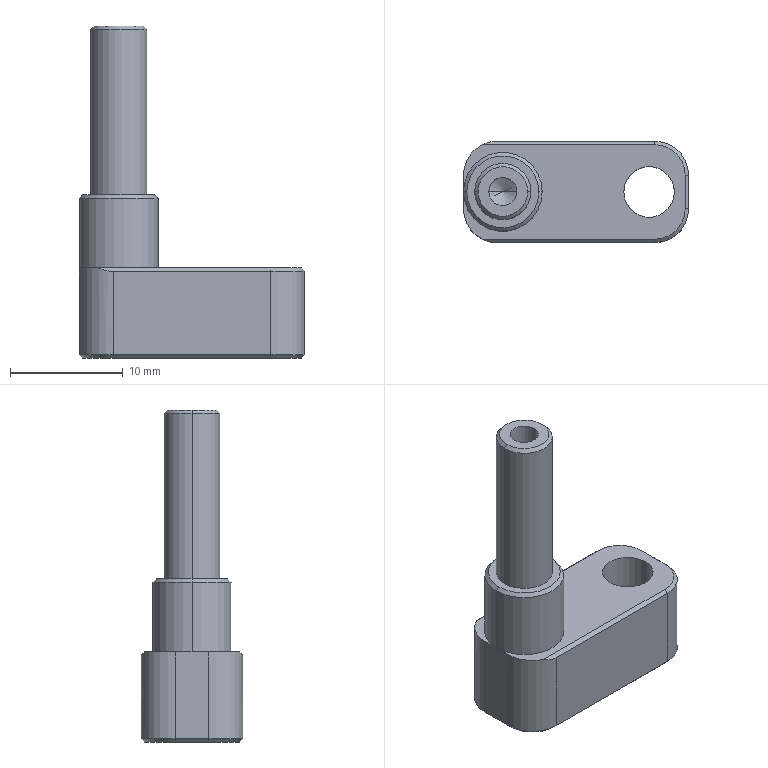Part | NX | features BREP 1 | 1 solid | 39 faces | box 20 x 9 x 29.5 mm | volume 1742 mm3 | plane 15 | cone 12 | cylinder 12 | commonest cylinder face diameters 6 x4 2.5 x2 4.5 x2 5 x2 7 x2
STEP:
#1=CARTESIAN_POINT('',(7.,4.2,8.));
#2=VERTEX_POINT('',#1);
#3=CARTESIAN_POINT('',(7.,4.5,7.7));
#4=VERTEX_POINT('',#3);
#5=CARTESIAN_POINT('',(7.,4.2,8.));
#6=DIRECTION('',(0.,0.7071,-0.7071));
#7=VECTOR('',#6,1000.);
#8=LINE('',#5,#7);
#9=EDGE_CURVE('',#2,#4,#8,.T.);
#10=ORIENTED_EDGE('',*,*,#9,.T.);
#11=CARTESIAN_POINT('',(-7.,4.5,7.7));
#12=VERTEX_POINT('',#11);
#13=CARTESIAN_POINT('',(7.,4.5,7.7));
#14=DIRECTION('',(1.,0.,0.));
#15=VECTOR('',#14,1000.);
#16=LINE('',#13,#15);
#17=EDGE_CURVE('',#12,#4,#16,.T.);
#18=ORIENTED_EDGE('',*,*,#17,.F.);
#19=CARTESIAN_POINT('',(-8.308,4.2,8.));
#20=VERTEX_POINT('',#19);
#21=CARTESIAN_POINT('',(-8.308,4.2,8.));
#22=CARTESIAN_POINT('',(-7.898,4.398,7.802));
#23=CARTESIAN_POINT('',(-7.455,4.5,7.7));
#24=CARTESIAN_POINT('',(-7.,4.5,7.7));
#25=(BOUNDED_CURVE()B_SPLINE_CURVE(3,(#21,#22,#23,#24),.UNSPECIFIED.,.F.,.F.)B_SPLINE_CURVE_WITH_KNOTS((4,4),(5.832,6.283),.UNSPECIFIED.)CURVE()GEOMETRIC_REPRESENTATION_ITEM()RATIONAL_B_SPLINE_CURVE((1.,0.9831,0.9831,1.))REPRESENTATION_ITEM(''));
#26=EDGE_CURVE('',#20,#12,#25,.T.);
#27=ORIENTED_EDGE('',*,*,#26,.F.);
#28=CARTESIAN_POINT('',(-7.,4.2,8.));
#29=DIRECTION('',(-1.,0.,0.));
#30=VECTOR('',#29,1000.);
#31=LINE('',#28,#30);
#32=EDGE_CURVE('',#2,#20,#31,.T.);
#33=ORIENTED_EDGE('',*,*,#32,.F.);
#34=EDGE_LOOP('',(#10,#18,#27,#33));
#35=FACE_BOUND('',#34,.T.);
#36=CARTESIAN_POINT('',(0.,4.2,8.));
#37=DIRECTION('',(0.,0.7071,0.7071));
#38=DIRECTION('',(1.,0.,0.));
#39=AXIS2_PLACEMENT_3D('',#36,#37,#38);
#40=PLANE('',#39);
#41=ADVANCED_FACE('',(#35),#40,.T.);
#42=CARTESIAN_POINT('',(9.7,1.5,8.));
#43=VERTEX_POINT('',#42);
#44=CARTESIAN_POINT('',(10.,1.5,7.7));
#45=VERTEX_POINT('',#44);
#46=CARTESIAN_POINT('',(9.7,1.5,8.));
#47=DIRECTION('',(0.7071,0.,-0.7071));
#48=VECTOR('',#47,1000.);
#49=LINE('',#46,#48);
#50=EDGE_CURVE('',#43,#45,#49,.T.);
#51=ORIENTED_EDGE('',*,*,#50,.T.);
#52=CARTESIAN_POINT('',(7.,1.5,7.7));
#53=DIRECTION('',(0.,0.,-1.));
#54=DIRECTION('',(1.,0.,0.));
#55=AXIS2_PLACEMENT_3D('',#52,#53,#54);
#56=CIRCLE('',#55,3.);
#57=EDGE_CURVE('',#4,#45,#56,.T.);
#58=ORIENTED_EDGE('',*,*,#57,.F.);
#59=ORIENTED_EDGE('',*,*,#9,.F.);
#60=CARTESIAN_POINT('',(7.,1.5,8.));
#61=DIRECTION('',(0.,0.,1.));
#62=DIRECTION('',(1.,0.,0.));
#63=AXIS2_PLACEMENT_3D('',#60,#61,#62);
#64=CIRCLE('',#63,2.7);
#65=EDGE_CURVE('',#43,#2,#64,.T.);
#66=ORIENTED_EDGE('',*,*,#65,.F.);
#67=EDGE_LOOP('',(#51,#58,#59,#66));
#68=FACE_BOUND('',#67,.T.);
#69=CARTESIAN_POINT('',(7.,1.5,8.));
#70=DIRECTION('',(0.,0.,-1.));
#71=DIRECTION('',(-1.,0.,0.));
#72=AXIS2_PLACEMENT_3D('',#69,#70,#71);
#73=CONICAL_SURFACE('',#72,2.7,0.7854);
#74=ADVANCED_FACE('',(#68),#73,.T.);
#75=CARTESIAN_POINT('',(9.7,-1.5,8.));
#76=VERTEX_POINT('',#75);
#77=CARTESIAN_POINT('',(10.,-1.5,7.7));
#78=VERTEX_POINT('',#77);
#79=CARTESIAN_POINT('',(9.7,-1.5,8.));
#80=DIRECTION('',(0.7071,0.,-0.7071));
#81=VECTOR('',#80,1000.);
#82=LINE('',#79,#81);
#83=EDGE_CURVE('',#76,#78,#82,.T.);
#84=ORIENTED_EDGE('',*,*,#83,.T.);
#85=CARTESIAN_POINT('',(10.,-1.5,7.7));
#86=DIRECTION('',(0.,-1.,0.));
#87=VECTOR('',#86,1000.);
#88=LINE('',#85,#87);
#89=EDGE_CURVE('',#45,#78,#88,.T.);
#90=ORIENTED_EDGE('',*,*,#89,.F.);
#91=ORIENTED_EDGE('',*,*,#50,.F.);
#92=CARTESIAN_POINT('',(9.7,1.5,8.));
#93=DIRECTION('',(0.,1.,0.));
#94=VECTOR('',#93,1000.);
#95=LINE('',#92,#94);
#96=EDGE_CURVE('',#76,#43,#95,.T.);
#97=ORIENTED_EDGE('',*,*,#96,.F.);
#98=EDGE_LOOP('',(#84,#90,#91,#97));
#99=FACE_BOUND('',#98,.T.);
#100=CARTESIAN_POINT('',(9.7,0.,8.));
#101=DIRECTION('',(0.7071,0.,0.7071));
#102=DIRECTION('',(0.,-1.,0.));
#103=AXIS2_PLACEMENT_3D('',#100,#101,#102);
#104=PLANE('',#103);
#105=ADVANCED_FACE('',(#99),#104,.T.);
#106=CARTESIAN_POINT('',(7.,-4.2,8.));
#107=VERTEX_POINT('',#106);
#108=CARTESIAN_POINT('',(7.,-4.5,7.7));
#109=VERTEX_POINT('',#108);
#110=CARTESIAN_POINT('',(7.,-4.2,8.));
#111=DIRECTION('',(0.,-0.7071,-0.7071));
#112=VECTOR('',#111,1000.);
#113=LINE('',#110,#112);
#114=EDGE_CURVE('',#107,#109,#113,.T.);
#115=ORIENTED_EDGE('',*,*,#114,.T.);
#116=CARTESIAN_POINT('',(7.,-1.5,7.7));
#117=DIRECTION('',(0.,0.,-1.));
#118=DIRECTION('',(1.,0.,0.));
#119=AXIS2_PLACEMENT_3D('',#116,#117,#118);
#120=CIRCLE('',#119,3.);
#121=EDGE_CURVE('',#78,#109,#120,.T.);
#122=ORIENTED_EDGE('',*,*,#121,.F.);
#123=ORIENTED_EDGE('',*,*,#83,.F.);
#124=CARTESIAN_POINT('',(7.,-1.5,8.));
#125=DIRECTION('',(0.,0.,1.));
#126=DIRECTION('',(1.,0.,0.));
#127=AXIS2_PLACEMENT_3D('',#124,#125,#126);
#128=CIRCLE('',#127,2.7);
#129=EDGE_CURVE('',#107,#76,#128,.T.);
#130=ORIENTED_EDGE('',*,*,#129,.F.);
#131=EDGE_LOOP('',(#115,#122,#123,#130));
#132=FACE_BOUND('',#131,.T.);
#133=CARTESIAN_POINT('',(7.,-1.5,8.));
#134=DIRECTION('',(0.,0.,-1.));
#135=DIRECTION('',(-1.,0.,0.));
#136=AXIS2_PLACEMENT_3D('',#133,#134,#135);
#137=CONICAL_SURFACE('',#136,2.7,0.7854);
#138=ADVANCED_FACE('',(#132),#137,.T.);
#139=CARTESIAN_POINT('',(-7.,-4.5,7.7));
#140=VERTEX_POINT('',#139);
#141=CARTESIAN_POINT('',(-8.308,-4.2,8.));
#142=VERTEX_POINT('',#141);
#143=CARTESIAN_POINT('',(-7.,-4.5,7.7));
#144=CARTESIAN_POINT('',(-7.455,-4.5,7.7));
#145=CARTESIAN_POINT('',(-7.898,-4.398,7.802));
#146=CARTESIAN_POINT('',(-8.308,-4.2,8.));
#147=(BOUNDED_CURVE()B_SPLINE_CURVE(3,(#143,#144,#145,#146),.UNSPECIFIED.,.F.,.F.)B_SPLINE_CURVE_WITH_KNOTS((4,4),(0.,0.451),.UNSPECIFIED.)CURVE()GEOMETRIC_REPRESENTATION_ITEM()RATIONAL_B_SPLINE_CURVE((1.,0.9831,0.9831,1.))REPRESENTATION_ITEM(''));
#148=EDGE_CURVE('',#140,#142,#147,.T.);
#149=ORIENTED_EDGE('',*,*,#148,.F.);
#150=CARTESIAN_POINT('',(-7.,-4.5,7.7));
#151=DIRECTION('',(-1.,0.,0.));
#152=VECTOR('',#151,1000.);
#153=LINE('',#150,#152);
#154=EDGE_CURVE('',#109,#140,#153,.T.);
#155=ORIENTED_EDGE('',*,*,#154,.F.);
#156=ORIENTED_EDGE('',*,*,#114,.F.);
#157=CARTESIAN_POINT('',(7.,-4.2,8.));
#158=DIRECTION('',(1.,0.,0.));
#159=VECTOR('',#158,1000.);
#160=LINE('',#157,#159);
#161=EDGE_CURVE('',#142,#107,#160,.T.);
#162=ORIENTED_EDGE('',*,*,#161,.F.);
#163=EDGE_LOOP('',(#149,#155,#156,#162));
#164=FACE_BOUND('',#163,.T.);
#165=CARTESIAN_POINT('',(0.,-4.2,8.));
#166=DIRECTION('',(0.,-0.7071,0.7071));
#167=DIRECTION('',(-1.,0.,0.));
#168=AXIS2_PLACEMENT_3D('',#165,#166,#167);
#169=PLANE('',#168);
#170=ADVANCED_FACE('',(#164),#169,.T.);
#171=CARTESIAN_POINT('',(-4.3,0.,29.5));
#172=VERTEX_POINT('',#171);
#173=CARTESIAN_POINT('',(-4.,0.,29.2));
#174=VERTEX_POINT('',#173);
#175=CARTESIAN_POINT('',(-4.3,0.,29.5));
#176=DIRECTION('',(0.7071,0.,-0.7071));
#177=VECTOR('',#176,1000.);
#178=LINE('',#175,#177);
#179=EDGE_CURVE('',#172,#174,#178,.T.);
#180=ORIENTED_EDGE('',*,*,#179,.F.);
#181=CARTESIAN_POINT('',(-8.7,0.,29.5));
#182=VERTEX_POINT('',#181);
#183=CARTESIAN_POINT('',(-6.5,0.,29.5));
#184=DIRECTION('',(0.,0.,1.));
#185=DIRECTION('',(1.,0.,0.));
#186=AXIS2_PLACEMENT_3D('',#183,#184,#185);
#187=CIRCLE('',#186,2.2);
#188=EDGE_CURVE('',#182,#172,#187,.T.);
#189=ORIENTED_EDGE('',*,*,#188,.F.);
#190=CARTESIAN_POINT('',(-9.,0.,29.2));
#191=VERTEX_POINT('',#190);
#192=CARTESIAN_POINT('',(-8.7,0.,29.5));
#193=DIRECTION('',(-0.7071,0.,-0.7071));
#194=VECTOR('',#193,1000.);
#195=LINE('',#192,#194);
#196=EDGE_CURVE('',#182,#191,#195,.T.);
#197=ORIENTED_EDGE('',*,*,#196,.T.);
#198=CARTESIAN_POINT('',(-6.5,0.,29.2));
#199=DIRECTION('',(0.,0.,-1.));
#200=DIRECTION('',(1.,0.,0.));
#201=AXIS2_PLACEMENT_3D('',#198,#199,#200);
#202=CIRCLE('',#201,2.5);
#203=EDGE_CURVE('',#174,#191,#202,.T.);
#204=ORIENTED_EDGE('',*,*,#203,.F.);
#205=EDGE_LOOP('',(#180,#189,#197,#204));
#206=FACE_BOUND('',#205,.T.);
#207=CARTESIAN_POINT('',(-6.5,0.,29.5));
#208=DIRECTION('',(0.,0.,-1.));
#209=DIRECTION('',(-1.,0.,0.));
#210=AXIS2_PLACEMENT_3D('',#207,#208,#209);
#211=CONICAL_SURFACE('',#210,2.2,0.7854);
#212=ADVANCED_FACE('',(#206),#211,.T.);
#213=CARTESIAN_POINT('',(-3.3,0.,14.5));
#214=VERTEX_POINT('',#213);
#215=CARTESIAN_POINT('',(-3.,0.,14.2));
#216=VERTEX_POINT('',#215);
#217=CARTESIAN_POINT('',(-3.3,0.,14.5));
#218=DIRECTION('',(0.7071,0.,-0.7071));
#219=VECTOR('',#218,1000.);
#220=LINE('',#217,#219);
#221=EDGE_CURVE('',#214,#216,#220,.T.);
#222=ORIENTED_EDGE('',*,*,#221,.F.);
#223=CARTESIAN_POINT('',(-9.7,0.,14.5));
#224=VERTEX_POINT('',#223);
#225=CARTESIAN_POINT('',(-6.5,0.,14.5));
#226=DIRECTION('',(0.,0.,1.));
#227=DIRECTION('',(1.,0.,0.));
#228=AXIS2_PLACEMENT_3D('',#225,#226,#227);
#229=CIRCLE('',#228,3.2);
#230=EDGE_CURVE('',#224,#214,#229,.T.);
#231=ORIENTED_EDGE('',*,*,#230,.F.);
#232=CARTESIAN_POINT('',(-10.,0.,14.2));
#233=VERTEX_POINT('',#232);
#234=CARTESIAN_POINT('',(-9.7,0.,14.5));
#235=DIRECTION('',(-0.7071,0.,-0.7071));
#236=VECTOR('',#235,1000.);
#237=LINE('',#234,#236);
#238=EDGE_CURVE('',#224,#233,#237,.T.);
#239=ORIENTED_EDGE('',*,*,#238,.T.);
#240=CARTESIAN_POINT('',(-6.5,0.,14.2));
#241=DIRECTION('',(0.,0.,-1.));
#242=DIRECTION('',(1.,0.,0.));
#243=AXIS2_PLACEMENT_3D('',#240,#241,#242);
#244=CIRCLE('',#243,3.5);
#245=EDGE_CURVE('',#216,#233,#244,.T.);
#246=ORIENTED_EDGE('',*,*,#245,.F.);
#247=EDGE_LOOP('',(#222,#231,#239,#246));
#248=FACE_BOUND('',#247,.T.);
#249=CARTESIAN_POINT('',(-6.5,0.,14.5));
#250=DIRECTION('',(0.,0.,-1.));
#251=DIRECTION('',(-1.,0.,0.));
#252=AXIS2_PLACEMENT_3D('',#249,#250,#251);
#253=CONICAL_SURFACE('',#252,3.2,0.7854);
#254=ADVANCED_FACE('',(#248),#253,.T.);
#255=CARTESIAN_POINT('',(7.,4.5,0.3));
#256=VERTEX_POINT('',#255);
#257=CARTESIAN_POINT('',(7.,4.2,0.));
#258=VERTEX_POINT('',#257);
#259=CARTESIAN_POINT('',(7.,4.5,0.3));
#260=DIRECTION('',(0.,-0.7071,-0.7071));
#261=VECTOR('',#260,1000.);
#262=LINE('',#259,#261);
#263=EDGE_CURVE('',#256,#258,#262,.T.);
#264=ORIENTED_EDGE('',*,*,#263,.T.);
#265=CARTESIAN_POINT('',(-7.,4.2,0.));
#266=VERTEX_POINT('',#265);
#267=CARTESIAN_POINT('',(0.,4.2,0.));
#268=DIRECTION('',(1.,0.,0.));
#269=VECTOR('',#268,1000.);
#270=LINE('',#267,#269);
#271=EDGE_CURVE('',#266,#258,#270,.T.);
#272=ORIENTED_EDGE('',*,*,#271,.F.);
#273=CARTESIAN_POINT('',(-7.,4.5,0.3));
#274=VERTEX_POINT('',#273);
#275=CARTESIAN_POINT('',(-7.,4.2,0.));
#276=DIRECTION('',(0.,0.7071,0.7071));
#277=VECTOR('',#276,1000.);
#278=LINE('',#275,#277);
#279=EDGE_CURVE('',#266,#274,#278,.T.);
#280=ORIENTED_EDGE('',*,*,#279,.T.);
#281=CARTESIAN_POINT('',(-10.,4.5,0.3));
#282=DIRECTION('',(-1.,0.,0.));
#283=VECTOR('',#282,1000.);
#284=LINE('',#281,#283);
#285=EDGE_CURVE('',#256,#274,#284,.T.);
#286=ORIENTED_EDGE('',*,*,#285,.F.);
#287=EDGE_LOOP('',(#264,#272,#280,#286));
#288=FACE_BOUND('',#287,.T.);
#289=CARTESIAN_POINT('',(-10.,4.5,0.3));
#290=DIRECTION('',(0.,-0.7071,0.7071));
#291=DIRECTION('',(-1.,0.,0.));
#292=AXIS2_PLACEMENT_3D('',#289,#290,#291);
#293=PLANE('',#292);
#294=ADVANCED_FACE('',(#288),#293,.F.);
#295=CARTESIAN_POINT('',(-9.7,1.5,0.));
#296=VERTEX_POINT('',#295);
#297=CARTESIAN_POINT('',(-10.,1.5,0.3));
#298=VERTEX_POINT('',#297);
#299=CARTESIAN_POINT('',(-9.7,1.5,0.));
#300=DIRECTION('',(-0.7071,0.,0.7071));
#301=VECTOR('',#300,1000.);
#302=LINE('',#299,#301);
#303=EDGE_CURVE('',#296,#298,#302,.T.);
#304=ORIENTED_EDGE('',*,*,#303,.T.);
#305=CARTESIAN_POINT('',(-7.,1.5,0.3));
#306=DIRECTION('',(0.,0.,1.));
#307=DIRECTION('',(1.,0.,0.));
#308=AXIS2_PLACEMENT_3D('',#305,#306,#307);
#309=CIRCLE('',#308,3.);
#310=EDGE_CURVE('',#274,#298,#309,.T.);
#311=ORIENTED_EDGE('',*,*,#310,.F.);
#312=ORIENTED_EDGE('',*,*,#279,.F.);
#313=CARTESIAN_POINT('',(-7.,1.5,0.));
#314=DIRECTION('',(0.,0.,-1.));
#315=DIRECTION('',(1.,0.,0.));
#316=AXIS2_PLACEMENT_3D('',#313,#314,#315);
#317=CIRCLE('',#316,2.7);
#318=EDGE_CURVE('',#296,#266,#317,.T.);
#319=ORIENTED_EDGE('',*,*,#318,.F.);
#320=EDGE_LOOP('',(#304,#311,#312,#319));
#321=FACE_BOUND('',#320,.T.);
#322=CARTESIAN_POINT('',(-7.,1.5,0.));
#323=DIRECTION('',(0.,0.,1.));
#324=DIRECTION('',(1.,0.,0.));
#325=AXIS2_PLACEMENT_3D('',#322,#323,#324);
#326=CONICAL_SURFACE('',#325,2.7,0.7854);
#327=ADVANCED_FACE('',(#321),#326,.T.);
#328=CARTESIAN_POINT('',(10.,1.5,0.3));
#329=VERTEX_POINT('',#328);
#330=CARTESIAN_POINT('',(9.7,1.5,0.));
#331=VERTEX_POINT('',#330);
#332=CARTESIAN_POINT('',(10.,1.5,0.3));
#333=DIRECTION('',(-0.7071,0.,-0.7071));
#334=VECTOR('',#333,1000.);
#335=LINE('',#332,#334);
#336=EDGE_CURVE('',#329,#331,#335,.T.);
#337=ORIENTED_EDGE('',*,*,#336,.T.);
#338=CARTESIAN_POINT('',(7.,1.5,0.));
#339=DIRECTION('',(0.,0.,-1.));
#340=DIRECTION('',(1.,0.,0.));
#341=AXIS2_PLACEMENT_3D('',#338,#339,#340);
#342=CIRCLE('',#341,2.7);
#343=EDGE_CURVE('',#258,#331,#342,.T.);
#344=ORIENTED_EDGE('',*,*,#343,.F.);
#345=ORIENTED_EDGE('',*,*,#263,.F.);
#346=CARTESIAN_POINT('',(7.,1.5,0.3));
#347=DIRECTION('',(0.,0.,1.));
#348=DIRECTION('',(1.,0.,0.));
#349=AXIS2_PLACEMENT_3D('',#346,#347,#348);
#350=CIRCLE('',#349,3.);
#351=EDGE_CURVE('',#329,#256,#350,.T.);
#352=ORIENTED_EDGE('',*,*,#351,.F.);
#353=EDGE_LOOP('',(#337,#344,#345,#352));
#354=FACE_BOUND('',#353,.T.);
#355=CARTESIAN_POINT('',(7.,1.5,0.));
#356=DIRECTION('',(0.,0.,1.));
#357=DIRECTION('',(1.,0.,0.));
#358=AXIS2_PLACEMENT_3D('',#355,#356,#357);
#359=CONICAL_SURFACE('',#358,2.7,0.7854);
#360=ADVANCED_FACE('',(#354),#359,.T.);
#361=CARTESIAN_POINT('',(-9.7,-1.5,0.));
#362=VERTEX_POINT('',#361);
#363=CARTESIAN_POINT('',(-10.,-1.5,0.3));
#364=VERTEX_POINT('',#363);
#365=CARTESIAN_POINT('',(-9.7,-1.5,0.));
#366=DIRECTION('',(-0.7071,0.,0.7071));
#367=VECTOR('',#366,1000.);
#368=LINE('',#365,#367);
#369=EDGE_CURVE('',#362,#364,#368,.T.);
#370=ORIENTED_EDGE('',*,*,#369,.T.);
#371=CARTESIAN_POINT('',(-10.,4.5,0.3));
#372=DIRECTION('',(0.,-1.,0.));
#373=VECTOR('',#372,1000.);
#374=LINE('',#371,#373);
#375=EDGE_CURVE('',#298,#364,#374,.T.);
#376=ORIENTED_EDGE('',*,*,#375,.F.);
#377=ORIENTED_EDGE('',*,*,#303,.F.);
#378=CARTESIAN_POINT('',(-9.7,0.,0.));
#379=DIRECTION('',(0.,1.,0.));
#380=VECTOR('',#379,1000.);
#381=LINE('',#378,#380);
#382=EDGE_CURVE('',#362,#296,#381,.T.);
#383=ORIENTED_EDGE('',*,*,#382,.F.);
#384=EDGE_LOOP('',(#370,#376,#377,#383));
#385=FACE_BOUND('',#384,.T.);
#386=CARTESIAN_POINT('',(-10.,4.5,0.3));
#387=DIRECTION('',(0.7071,0.,0.7071));
#388=DIRECTION('',(0.,-1.,0.));
#389=AXIS2_PLACEMENT_3D('',#386,#387,#388);
#390=PLANE('',#389);
#391=ADVANCED_FACE('',(#385),#390,.F.);
#392=CARTESIAN_POINT('',(10.,-1.5,0.3));
#393=VERTEX_POINT('',#392);
#394=CARTESIAN_POINT('',(9.7,-1.5,0.));
#395=VERTEX_POINT('',#394);
#396=CARTESIAN_POINT('',(10.,-1.5,0.3));
#397=DIRECTION('',(-0.7071,0.,-0.7071));
#398=VECTOR('',#397,1000.);
#399=LINE('',#396,#398);
#400=EDGE_CURVE('',#393,#395,#399,.T.);
#401=ORIENTED_EDGE('',*,*,#400,.T.);
#402=CARTESIAN_POINT('',(9.7,0.,0.));
#403=DIRECTION('',(0.,-1.,0.));
#404=VECTOR('',#403,1000.);
#405=LINE('',#402,#404);
#406=EDGE_CURVE('',#331,#395,#405,.T.);
#407=ORIENTED_EDGE('',*,*,#406,.F.);
#408=ORIENTED_EDGE('',*,*,#336,.F.);
#409=CARTESIAN_POINT('',(10.,4.5,0.3));
#410=DIRECTION('',(0.,1.,0.));
#411=VECTOR('',#410,1000.);
#412=LINE('',#409,#411);
#413=EDGE_CURVE('',#393,#329,#412,.T.);
#414=ORIENTED_EDGE('',*,*,#413,.F.);
#415=EDGE_LOOP('',(#401,#407,#408,#414));
#416=FACE_BOUND('',#415,.T.);
#417=CARTESIAN_POINT('',(10.,4.5,0.3));
#418=DIRECTION('',(-0.7071,0.,0.7071));
#419=DIRECTION('',(0.,1.,0.));
#420=AXIS2_PLACEMENT_3D('',#417,#418,#419);
#421=PLANE('',#420);
#422=ADVANCED_FACE('',(#416),#421,.F.);
#423=CARTESIAN_POINT('',(-7.,-4.2,0.));
#424=VERTEX_POINT('',#423);
#425=CARTESIAN_POINT('',(-7.,-4.5,0.3));
#426=VERTEX_POINT('',#425);
#427=CARTESIAN_POINT('',(-7.,-4.2,0.));
#428=DIRECTION('',(0.,-0.7071,0.7071));
#429=VECTOR('',#428,1000.);
#430=LINE('',#427,#429);
#431=EDGE_CURVE('',#424,#426,#430,.T.);
#432=ORIENTED_EDGE('',*,*,#431,.T.);
#433=CARTESIAN_POINT('',(-7.,-1.5,0.3));
#434=DIRECTION('',(0.,0.,1.));
#435=DIRECTION('',(1.,0.,0.));
#436=AXIS2_PLACEMENT_3D('',#433,#434,#435);
#437=CIRCLE('',#436,3.);
#438=EDGE_CURVE('',#364,#426,#437,.T.);
#439=ORIENTED_EDGE('',*,*,#438,.F.);
#440=ORIENTED_EDGE('',*,*,#369,.F.);
#441=CARTESIAN_POINT('',(-7.,-1.5,0.));
#442=DIRECTION('',(0.,0.,-1.));
#443=DIRECTION('',(1.,0.,0.));
#444=AXIS2_PLACEMENT_3D('',#441,#442,#443);
#445=CIRCLE('',#444,2.7);
#446=EDGE_CURVE('',#424,#362,#445,.T.);
#447=ORIENTED_EDGE('',*,*,#446,.F.);
#448=EDGE_LOOP('',(#432,#439,#440,#447));
#449=FACE_BOUND('',#448,.T.);
#450=CARTESIAN_POINT('',(-7.,-1.5,0.));
#451=DIRECTION('',(0.,0.,1.));
#452=DIRECTION('',(1.,0.,0.));
#453=AXIS2_PLACEMENT_3D('',#450,#451,#452);
#454=CONICAL_SURFACE('',#453,2.7,0.7854);
#455=ADVANCED_FACE('',(#449),#454,.T.);
#456=CARTESIAN_POINT('',(7.,-4.5,0.3));
#457=VERTEX_POINT('',#456);
#458=CARTESIAN_POINT('',(7.,-4.2,0.));
#459=VERTEX_POINT('',#458);
#460=CARTESIAN_POINT('',(7.,-4.5,0.3));
#461=DIRECTION('',(0.,0.7071,-0.7071));
#462=VECTOR('',#461,1000.);
#463=LINE('',#460,#462);
#464=EDGE_CURVE('',#457,#459,#463,.T.);
#465=ORIENTED_EDGE('',*,*,#464,.T.);
#466=CARTESIAN_POINT('',(7.,-1.5,0.));
#467=DIRECTION('',(0.,0.,-1.));
#468=DIRECTION('',(1.,0.,0.));
#469=AXIS2_PLACEMENT_3D('',#466,#467,#468);
#470=CIRCLE('',#469,2.7);
#471=EDGE_CURVE('',#395,#459,#470,.T.);
#472=ORIENTED_EDGE('',*,*,#471,.F.);
#473=ORIENTED_EDGE('',*,*,#400,.F.);
#474=CARTESIAN_POINT('',(7.,-1.5,0.3));
#475=DIRECTION('',(0.,0.,1.));
#476=DIRECTION('',(1.,0.,0.));
#477=AXIS2_PLACEMENT_3D('',#474,#475,#476);
#478=CIRCLE('',#477,3.);
#479=EDGE_CURVE('',#457,#393,#478,.T.);
#480=ORIENTED_EDGE('',*,*,#479,.F.);
#481=EDGE_LOOP('',(#465,#472,#473,#480));
#482=FACE_BOUND('',#481,.T.);
#483=CARTESIAN_POINT('',(7.,-1.5,0.));
#484=DIRECTION('',(0.,0.,1.));
#485=DIRECTION('',(1.,0.,0.));
#486=AXIS2_PLACEMENT_3D('',#483,#484,#485);
#487=CONICAL_SURFACE('',#486,2.7,0.7854);
#488=ADVANCED_FACE('',(#482),#487,.T.);
#489=ORIENTED_EDGE('',*,*,#431,.F.);
#490=CARTESIAN_POINT('',(0.,-4.2,0.));
#491=DIRECTION('',(-1.,0.,0.));
#492=VECTOR('',#491,1000.);
#493=LINE('',#490,#492);
#494=EDGE_CURVE('',#459,#424,#493,.T.);
#495=ORIENTED_EDGE('',*,*,#494,.F.);
#496=ORIENTED_EDGE('',*,*,#464,.F.);
#497=CARTESIAN_POINT('',(-10.,-4.5,0.3));
#498=DIRECTION('',(1.,0.,0.));
#499=VECTOR('',#498,1000.);
#500=LINE('',#497,#499);
#501=EDGE_CURVE('',#426,#457,#500,.T.);
#502=ORIENTED_EDGE('',*,*,#501,.F.);
#503=EDGE_LOOP('',(#489,#495,#496,#502));
#504=FACE_BOUND('',#503,.T.);
#505=CARTESIAN_POINT('',(-10.,-4.5,0.3));
#506=DIRECTION('',(0.,0.7071,0.7071));
#507=DIRECTION('',(1.,0.,0.));
#508=AXIS2_PLACEMENT_3D('',#505,#506,#507);
#509=PLANE('',#508);
#510=ADVANCED_FACE('',(#504),#509,.F.);
#511=CARTESIAN_POINT('',(-7.,-4.5,8.));
#512=DIRECTION('',(0.,0.,-1.));
#513=VECTOR('',#512,1000.);
#514=LINE('',#511,#513);
#515=EDGE_CURVE('',#140,#426,#514,.T.);
#516=ORIENTED_EDGE('',*,*,#515,.F.);
#517=ORIENTED_EDGE('',*,*,#148,.T.);
#518=CARTESIAN_POINT('',(-10.,-1.5,8.));
#519=VERTEX_POINT('',#518);
#520=CARTESIAN_POINT('',(-7.,-1.5,8.));
#521=DIRECTION('',(0.,0.,1.));
#522=DIRECTION('',(1.,0.,0.));
#523=AXIS2_PLACEMENT_3D('',#520,#521,#522);
#524=CIRCLE('',#523,3.);
#525=EDGE_CURVE('',#519,#142,#524,.T.);
#526=ORIENTED_EDGE('',*,*,#525,.F.);
#527=CARTESIAN_POINT('',(-10.,-1.5,8.));
#528=DIRECTION('',(0.,0.,1.));
#529=VECTOR('',#528,1000.);
#530=LINE('',#527,#529);
#531=EDGE_CURVE('',#364,#519,#530,.T.);
#532=ORIENTED_EDGE('',*,*,#531,.F.);
#533=ORIENTED_EDGE('',*,*,#438,.T.);
#534=EDGE_LOOP('',(#516,#517,#526,#532,#533));
#535=FACE_BOUND('',#534,.T.);
#536=CARTESIAN_POINT('',(-7.,-1.5,8.));
#537=DIRECTION('',(0.,0.,-1.));
#538=DIRECTION('',(-1.,0.,0.));
#539=AXIS2_PLACEMENT_3D('',#536,#537,#538);
#540=CYLINDRICAL_SURFACE('',#539,3.);
#541=ADVANCED_FACE('',(#535),#540,.T.);
#542=CARTESIAN_POINT('',(10.,-1.5,8.));
#543=DIRECTION('',(0.,0.,-1.));
#544=VECTOR('',#543,1000.);
#545=LINE('',#542,#544);
#546=EDGE_CURVE('',#78,#393,#545,.T.);
#547=ORIENTED_EDGE('',*,*,#546,.F.);
#548=ORIENTED_EDGE('',*,*,#121,.T.);
#549=CARTESIAN_POINT('',(7.,-4.5,8.));
#550=DIRECTION('',(0.,0.,1.));
#551=VECTOR('',#550,1000.);
#552=LINE('',#549,#551);
#553=EDGE_CURVE('',#457,#109,#552,.T.);
#554=ORIENTED_EDGE('',*,*,#553,.F.);
#555=ORIENTED_EDGE('',*,*,#479,.T.);
#556=EDGE_LOOP('',(#547,#548,#554,#555));
#557=FACE_BOUND('',#556,.T.);
#558=CARTESIAN_POINT('',(7.,-1.5,8.));
#559=DIRECTION('',(0.,0.,-1.));
#560=DIRECTION('',(-1.,0.,0.));
#561=AXIS2_PLACEMENT_3D('',#558,#559,#560);
#562=CYLINDRICAL_SURFACE('',#561,3.);
#563=ADVANCED_FACE('',(#557),#562,.T.);
#564=CARTESIAN_POINT('',(7.,4.5,8.));
#565=DIRECTION('',(0.,0.,-1.));
#566=VECTOR('',#565,1000.);
#567=LINE('',#564,#566);
#568=EDGE_CURVE('',#4,#256,#567,.T.);
#569=ORIENTED_EDGE('',*,*,#568,.F.);
#570=ORIENTED_EDGE('',*,*,#57,.T.);
#571=CARTESIAN_POINT('',(10.,1.5,8.));
#572=DIRECTION('',(0.,0.,1.));
#573=VECTOR('',#572,1000.);
#574=LINE('',#571,#573);
#575=EDGE_CURVE('',#329,#45,#574,.T.);
#576=ORIENTED_EDGE('',*,*,#575,.F.);
#577=ORIENTED_EDGE('',*,*,#351,.T.);
#578=EDGE_LOOP('',(#569,#570,#576,#577));
#579=FACE_BOUND('',#578,.T.);
#580=CARTESIAN_POINT('',(7.,1.5,8.));
#581=DIRECTION('',(0.,0.,-1.));
#582=DIRECTION('',(-1.,0.,0.));
#583=AXIS2_PLACEMENT_3D('',#580,#581,#582);
#584=CYLINDRICAL_SURFACE('',#583,3.);
#585=ADVANCED_FACE('',(#579),#584,.T.);
#586=CARTESIAN_POINT('',(-10.,1.5,8.));
#587=VERTEX_POINT('',#586);
#588=CARTESIAN_POINT('',(-7.,1.5,8.));
#589=DIRECTION('',(0.,0.,1.));
#590=DIRECTION('',(1.,0.,0.));
#591=AXIS2_PLACEMENT_3D('',#588,#589,#590);
#592=CIRCLE('',#591,3.);
#593=EDGE_CURVE('',#20,#587,#592,.T.);
#594=ORIENTED_EDGE('',*,*,#593,.F.);
#595=ORIENTED_EDGE('',*,*,#26,.T.);
#596=CARTESIAN_POINT('',(-7.,4.5,8.));
#597=DIRECTION('',(0.,0.,1.));
#598=VECTOR('',#597,1000.);
#599=LINE('',#596,#598);
#600=EDGE_CURVE('',#274,#12,#599,.T.);
#601=ORIENTED_EDGE('',*,*,#600,.F.);
#602=ORIENTED_EDGE('',*,*,#310,.T.);
#603=CARTESIAN_POINT('',(-10.,1.5,8.));
#604=DIRECTION('',(0.,0.,-1.));
#605=VECTOR('',#604,1000.);
#606=LINE('',#603,#605);
#607=EDGE_CURVE('',#587,#298,#606,.T.);
#608=ORIENTED_EDGE('',*,*,#607,.F.);
#609=EDGE_LOOP('',(#594,#595,#601,#602,#608));
#610=FACE_BOUND('',#609,.T.);
#611=CARTESIAN_POINT('',(-7.,1.5,8.));
#612=DIRECTION('',(0.,0.,-1.));
#613=DIRECTION('',(-1.,0.,0.));
#614=AXIS2_PLACEMENT_3D('',#611,#612,#613);
#615=CYLINDRICAL_SURFACE('',#614,3.);
#616=ADVANCED_FACE('',(#610),#615,.T.);
#617=CARTESIAN_POINT('',(-7.75,0.,29.5));
#618=VERTEX_POINT('',#617);
#619=CARTESIAN_POINT('',(-7.75,0.,20.));
#620=VERTEX_POINT('',#619);
#621=CARTESIAN_POINT('',(-7.75,0.,29.5));
#622=DIRECTION('',(0.,0.,1.));
#623=VECTOR('',#622,1000.);
#624=LINE('',#621,#623);
#625=EDGE_CURVE('',#618,#620,#624,.F.);
#626=ORIENTED_EDGE('',*,*,#625,.T.);
#627=CARTESIAN_POINT('',(-5.25,0.,20.));
#628=VERTEX_POINT('',#627);
#629=CARTESIAN_POINT('',(-6.5,0.,20.));
#630=DIRECTION('',(0.,0.,1.));
#631=DIRECTION('',(1.,0.,0.));
#632=AXIS2_PLACEMENT_3D('',#629,#630,#631);
#633=CIRCLE('',#632,1.25);
#634=EDGE_CURVE('',#628,#620,#633,.T.);
#635=ORIENTED_EDGE('',*,*,#634,.F.);
#636=CARTESIAN_POINT('',(-5.25,0.,29.5));
#637=VERTEX_POINT('',#636);
#638=CARTESIAN_POINT('',(-5.25,0.,29.5));
#639=DIRECTION('',(0.,0.,1.));
#640=VECTOR('',#639,1000.);
#641=LINE('',#638,#640);
#642=EDGE_CURVE('',#637,#628,#641,.F.);
#643=ORIENTED_EDGE('',*,*,#642,.F.);
#644=CARTESIAN_POINT('',(-6.5,0.,29.5));
#645=DIRECTION('',(0.,0.,1.));
#646=DIRECTION('',(1.,0.,0.));
#647=AXIS2_PLACEMENT_3D('',#644,#645,#646);
#648=CIRCLE('',#647,1.25);
#649=EDGE_CURVE('',#637,#618,#648,.T.);
#650=ORIENTED_EDGE('',*,*,#649,.T.);
#651=EDGE_LOOP('',(#626,#635,#643,#650));
#652=FACE_BOUND('',#651,.T.);
#653=CARTESIAN_POINT('',(-6.5,0.,29.5));
#654=DIRECTION('',(0.,0.,1.));
#655=DIRECTION('',(1.,0.,0.));
#656=AXIS2_PLACEMENT_3D('',#653,#654,#655);
#657=CYLINDRICAL_SURFACE('',#656,1.25);
#658=ADVANCED_FACE('',(#652),#657,.F.);
#659=CARTESIAN_POINT('',(-6.5,0.,19.249));
#660=VERTEX_POINT('',#659);
#661=CARTESIAN_POINT('',(-7.75,0.,20.));
#662=DIRECTION('',(-0.8572,0.,0.515));
#663=VECTOR('',#662,1000.);
#664=LINE('',#661,#663);
#665=EDGE_CURVE('',#660,#620,#664,.T.);
#666=ORIENTED_EDGE('',*,*,#665,.F.);
#667=CARTESIAN_POINT('',(-5.25,0.,20.));
#668=DIRECTION('',(0.8572,0.,0.515));
#669=VECTOR('',#668,1000.);
#670=LINE('',#667,#669);
#671=EDGE_CURVE('',#660,#628,#670,.T.);
#672=ORIENTED_EDGE('',*,*,#671,.T.);
#673=ORIENTED_EDGE('',*,*,#634,.T.);
#674=EDGE_LOOP('',(#666,#672,#673));
#675=FACE_BOUND('',#674,.T.);
#676=CARTESIAN_POINT('',(-6.5,0.,20.));
#677=DIRECTION('',(0.,0.,1.));
#678=DIRECTION('',(1.,0.,0.));
#679=AXIS2_PLACEMENT_3D('',#676,#677,#678);
#680=CONICAL_SURFACE('',#679,1.25,1.03);
#681=ADVANCED_FACE('',(#675),#680,.F.);
#682=CARTESIAN_POINT('',(4.25,0.,8.));
#683=VERTEX_POINT('',#682);
#684=CARTESIAN_POINT('',(4.25,0.,0.));
#685=VERTEX_POINT('',#684);
#686=CARTESIAN_POINT('',(4.25,0.,-7.));
#687=DIRECTION('',(0.,0.,1.));
#688=VECTOR('',#687,1000.);
#689=LINE('',#686,#688);
#690=EDGE_CURVE('',#683,#685,#689,.F.);
#691=ORIENTED_EDGE('',*,*,#690,.T.);
#692=CARTESIAN_POINT('',(8.75,0.,0.));
#693=VERTEX_POINT('',#692);
#694=CARTESIAN_POINT('',(6.5,0.,0.));
#695=DIRECTION('',(0.,0.,1.));
#696=DIRECTION('',(1.,0.,0.));
#697=AXIS2_PLACEMENT_3D('',#694,#695,#696);
#698=CIRCLE('',#697,2.25);
#699=EDGE_CURVE('',#693,#685,#698,.T.);
#700=ORIENTED_EDGE('',*,*,#699,.F.);
#701=CARTESIAN_POINT('',(8.75,0.,8.));
#702=VERTEX_POINT('',#701);
#703=CARTESIAN_POINT('',(8.75,0.,-7.));
#704=DIRECTION('',(0.,0.,1.));
#705=VECTOR('',#704,1000.);
#706=LINE('',#703,#705);
#707=EDGE_CURVE('',#702,#693,#706,.F.);
#708=ORIENTED_EDGE('',*,*,#707,.F.);
#709=CARTESIAN_POINT('',(6.5,0.,8.));
#710=DIRECTION('',(0.,0.,1.));
#711=DIRECTION('',(1.,0.,0.));
#712=AXIS2_PLACEMENT_3D('',#709,#710,#711);
#713=CIRCLE('',#712,2.25);
#714=EDGE_CURVE('',#702,#683,#713,.T.);
#715=ORIENTED_EDGE('',*,*,#714,.T.);
#716=EDGE_LOOP('',(#691,#700,#708,#715));
#717=FACE_BOUND('',#716,.T.);
#718=CARTESIAN_POINT('',(6.5,0.,-7.));
#719=DIRECTION('',(0.,0.,1.));
#720=DIRECTION('',(1.,0.,0.));
#721=AXIS2_PLACEMENT_3D('',#718,#719,#720);
#722=CYLINDRICAL_SURFACE('',#721,2.25);
#723=ADVANCED_FACE('',(#717),#722,.F.);
#724=ORIENTED_EDGE('',*,*,#649,.F.);
#725=CARTESIAN_POINT('',(-6.5,0.,29.5));
#726=DIRECTION('',(0.,0.,1.));
#727=DIRECTION('',(1.,0.,0.));
#728=AXIS2_PLACEMENT_3D('',#725,#726,#727);
#729=CIRCLE('',#728,1.25);
#730=EDGE_CURVE('',#618,#637,#729,.T.);
#731=ORIENTED_EDGE('',*,*,#730,.F.);
#732=EDGE_LOOP('',(#724,#731));
#733=FACE_BOUND('',#732,.T.);
#734=ORIENTED_EDGE('',*,*,#188,.T.);
#735=CARTESIAN_POINT('',(-6.5,0.,29.5));
#736=DIRECTION('',(0.,0.,1.));
#737=DIRECTION('',(1.,0.,0.));
#738=AXIS2_PLACEMENT_3D('',#735,#736,#737);
#739=CIRCLE('',#738,2.2);
#740=EDGE_CURVE('',#172,#182,#739,.T.);
#741=ORIENTED_EDGE('',*,*,#740,.T.);
#742=EDGE_LOOP('',(#734,#741));
#743=FACE_BOUND('',#742,.T.);
#744=CARTESIAN_POINT('',(-6.5,0.,29.5));
#745=DIRECTION('',(0.,0.,1.));
#746=DIRECTION('',(1.,0.,0.));
#747=AXIS2_PLACEMENT_3D('',#744,#745,#746);
#748=PLANE('',#747);
#749=ADVANCED_FACE('',(#733,#743),#748,.T.);
#750=CARTESIAN_POINT('',(-4.,0.,14.5));
#751=VERTEX_POINT('',#750);
#752=CARTESIAN_POINT('',(-4.,0.,29.5));
#753=DIRECTION('',(0.,0.,-1.));
#754=VECTOR('',#753,1000.);
#755=LINE('',#752,#754);
#756=EDGE_CURVE('',#174,#751,#755,.T.);
#757=ORIENTED_EDGE('',*,*,#756,.F.);
#758=ORIENTED_EDGE('',*,*,#203,.T.);
#759=CARTESIAN_POINT('',(-9.,0.,14.5));
#760=VERTEX_POINT('',#759);
#761=CARTESIAN_POINT('',(-9.,0.,29.5));
#762=DIRECTION('',(0.,0.,-1.));
#763=VECTOR('',#762,1000.);
#764=LINE('',#761,#763);
#765=EDGE_CURVE('',#191,#760,#764,.T.);
#766=ORIENTED_EDGE('',*,*,#765,.T.);
#767=CARTESIAN_POINT('',(-6.5,0.,14.5));
#768=DIRECTION('',(0.,0.,1.));
#769=DIRECTION('',(1.,0.,0.));
#770=AXIS2_PLACEMENT_3D('',#767,#768,#769);
#771=CIRCLE('',#770,2.5);
#772=EDGE_CURVE('',#760,#751,#771,.T.);
#773=ORIENTED_EDGE('',*,*,#772,.T.);
#774=EDGE_LOOP('',(#757,#758,#766,#773));
#775=FACE_BOUND('',#774,.T.);
#776=CARTESIAN_POINT('',(-6.5,0.,29.5));
#777=DIRECTION('',(0.,0.,-1.));
#778=DIRECTION('',(-1.,0.,0.));
#779=AXIS2_PLACEMENT_3D('',#776,#777,#778);
#780=CYLINDRICAL_SURFACE('',#779,2.5);
#781=ADVANCED_FACE('',(#775),#780,.T.);
#782=ORIENTED_EDGE('',*,*,#772,.F.);
#783=CARTESIAN_POINT('',(-6.5,0.,14.5));
#784=DIRECTION('',(0.,0.,1.));
#785=DIRECTION('',(1.,0.,0.));
#786=AXIS2_PLACEMENT_3D('',#783,#784,#785);
#787=CIRCLE('',#786,2.5);
#788=EDGE_CURVE('',#751,#760,#787,.T.);
#789=ORIENTED_EDGE('',*,*,#788,.F.);
#790=EDGE_LOOP('',(#782,#789));
#791=FACE_BOUND('',#790,.T.);
#792=ORIENTED_EDGE('',*,*,#230,.T.);
#793=CARTESIAN_POINT('',(-6.5,0.,14.5));
#794=DIRECTION('',(0.,0.,1.));
#795=DIRECTION('',(1.,0.,0.));
#796=AXIS2_PLACEMENT_3D('',#793,#794,#795);
#797=CIRCLE('',#796,3.2);
#798=EDGE_CURVE('',#214,#224,#797,.T.);
#799=ORIENTED_EDGE('',*,*,#798,.T.);
#800=EDGE_LOOP('',(#792,#799));
#801=FACE_BOUND('',#800,.T.);
#802=CARTESIAN_POINT('',(-6.5,0.,14.5));
#803=DIRECTION('',(0.,0.,1.));
#804=DIRECTION('',(1.,0.,0.));
#805=AXIS2_PLACEMENT_3D('',#802,#803,#804);
#806=PLANE('',#805);
#807=ADVANCED_FACE('',(#791,#801),#806,.T.);
#808=CARTESIAN_POINT('',(-3.,0.,8.));
#809=VERTEX_POINT('',#808);
#810=CARTESIAN_POINT('',(-3.,0.,14.5));
#811=DIRECTION('',(0.,0.,-1.));
#812=VECTOR('',#811,1000.);
#813=LINE('',#810,#812);
#814=EDGE_CURVE('',#216,#809,#813,.T.);
#815=ORIENTED_EDGE('',*,*,#814,.F.);
#816=ORIENTED_EDGE('',*,*,#245,.T.);
#817=CARTESIAN_POINT('',(-10.,0.,8.));
#818=VERTEX_POINT('',#817);
#819=CARTESIAN_POINT('',(-10.,0.,14.5));
#820=DIRECTION('',(0.,0.,-1.));
#821=VECTOR('',#820,1000.);
#822=LINE('',#819,#821);
#823=EDGE_CURVE('',#233,#818,#822,.T.);
#824=ORIENTED_EDGE('',*,*,#823,.T.);
#825=CARTESIAN_POINT('',(-6.5,0.,8.));
#826=DIRECTION('',(0.,0.,1.));
#827=DIRECTION('',(1.,0.,0.));
#828=AXIS2_PLACEMENT_3D('',#825,#826,#827);
#829=CIRCLE('',#828,3.5);
#830=EDGE_CURVE('',#818,#809,#829,.T.);
#831=ORIENTED_EDGE('',*,*,#830,.T.);
#832=EDGE_LOOP('',(#815,#816,#824,#831));
#833=FACE_BOUND('',#832,.T.);
#834=CARTESIAN_POINT('',(-6.5,0.,14.5));
#835=DIRECTION('',(0.,0.,-1.));
#836=DIRECTION('',(-1.,0.,0.));
#837=AXIS2_PLACEMENT_3D('',#834,#835,#836);
#838=CYLINDRICAL_SURFACE('',#837,3.5);
#839=ADVANCED_FACE('',(#833),#838,.T.);
#840=ORIENTED_EDGE('',*,*,#699,.T.);
#841=CARTESIAN_POINT('',(6.5,0.,0.));
#842=DIRECTION('',(0.,0.,1.));
#843=DIRECTION('',(1.,0.,0.));
#844=AXIS2_PLACEMENT_3D('',#841,#842,#843);
#845=CIRCLE('',#844,2.25);
#846=EDGE_CURVE('',#685,#693,#845,.T.);
#847=ORIENTED_EDGE('',*,*,#846,.T.);
#848=EDGE_LOOP('',(#840,#847));
#849=FACE_BOUND('',#848,.T.);
#850=ORIENTED_EDGE('',*,*,#318,.T.);
#851=ORIENTED_EDGE('',*,*,#271,.T.);
#852=ORIENTED_EDGE('',*,*,#343,.T.);
#853=ORIENTED_EDGE('',*,*,#406,.T.);
#854=ORIENTED_EDGE('',*,*,#471,.T.);
#855=ORIENTED_EDGE('',*,*,#494,.T.);
#856=ORIENTED_EDGE('',*,*,#446,.T.);
#857=ORIENTED_EDGE('',*,*,#382,.T.);
#858=EDGE_LOOP('',(#850,#851,#852,#853,#854,#855,#856,#857));
#859=FACE_BOUND('',#858,.T.);
#860=CARTESIAN_POINT('',(0.,0.,0.));
#861=DIRECTION('',(0.,0.,1.));
#862=DIRECTION('',(1.,0.,0.));
#863=AXIS2_PLACEMENT_3D('',#860,#861,#862);
#864=PLANE('',#863);
#865=ADVANCED_FACE('',(#849,#859),#864,.F.);
#866=ORIENTED_EDGE('',*,*,#65,.T.);
#867=ORIENTED_EDGE('',*,*,#32,.T.);
#868=ORIENTED_EDGE('',*,*,#593,.T.);
#869=CARTESIAN_POINT('',(-10.,4.5,8.));
#870=DIRECTION('',(0.,-1.,0.));
#871=VECTOR('',#870,1000.);
#872=LINE('',#869,#871);
#873=EDGE_CURVE('',#587,#818,#872,.T.);
#874=ORIENTED_EDGE('',*,*,#873,.T.);
#875=CARTESIAN_POINT('',(-6.5,0.,8.));
#876=DIRECTION('',(0.,0.,1.));
#877=DIRECTION('',(1.,0.,0.));
#878=AXIS2_PLACEMENT_3D('',#875,#876,#877);
#879=CIRCLE('',#878,3.5);
#880=EDGE_CURVE('',#809,#818,#879,.T.);
#881=ORIENTED_EDGE('',*,*,#880,.F.);
#882=ORIENTED_EDGE('',*,*,#830,.F.);
#883=CARTESIAN_POINT('',(-10.,4.5,8.));
#884=DIRECTION('',(0.,-1.,0.));
#885=VECTOR('',#884,1000.);
#886=LINE('',#883,#885);
#887=EDGE_CURVE('',#818,#519,#886,.T.);
#888=ORIENTED_EDGE('',*,*,#887,.T.);
#889=ORIENTED_EDGE('',*,*,#525,.T.);
#890=ORIENTED_EDGE('',*,*,#161,.T.);
#891=ORIENTED_EDGE('',*,*,#129,.T.);
#892=ORIENTED_EDGE('',*,*,#96,.T.);
#893=EDGE_LOOP('',(#866,#867,#868,#874,#881,#882,#888,#889,#890,#891,#892));
#894=FACE_BOUND('',#893,.T.);
#895=ORIENTED_EDGE('',*,*,#714,.F.);
#896=CARTESIAN_POINT('',(6.5,0.,8.));
#897=DIRECTION('',(0.,0.,1.));
#898=DIRECTION('',(1.,0.,0.));
#899=AXIS2_PLACEMENT_3D('',#896,#897,#898);
#900=CIRCLE('',#899,2.25);
#901=EDGE_CURVE('',#683,#702,#900,.T.);
#902=ORIENTED_EDGE('',*,*,#901,.F.);
#903=EDGE_LOOP('',(#895,#902));
#904=FACE_BOUND('',#903,.T.);
#905=CARTESIAN_POINT('',(0.,0.,8.));
#906=DIRECTION('',(0.,0.,1.));
#907=DIRECTION('',(1.,0.,0.));
#908=AXIS2_PLACEMENT_3D('',#905,#906,#907);
#909=PLANE('',#908);
#910=ADVANCED_FACE('',(#894,#904),#909,.T.);
#911=ORIENTED_EDGE('',*,*,#553,.T.);
#912=ORIENTED_EDGE('',*,*,#154,.T.);
#913=ORIENTED_EDGE('',*,*,#515,.T.);
#914=ORIENTED_EDGE('',*,*,#501,.T.);
#915=EDGE_LOOP('',(#911,#912,#913,#914));
#916=FACE_BOUND('',#915,.T.);
#917=CARTESIAN_POINT('',(-10.,-4.5,8.));
#918=DIRECTION('',(0.,1.,0.));
#919=DIRECTION('',(0.,0.,1.));
#920=AXIS2_PLACEMENT_3D('',#917,#918,#919);
#921=PLANE('',#920);
#922=ADVANCED_FACE('',(#916),#921,.F.);
#923=ORIENTED_EDGE('',*,*,#607,.T.);
#924=ORIENTED_EDGE('',*,*,#375,.T.);
#925=ORIENTED_EDGE('',*,*,#531,.T.);
#926=ORIENTED_EDGE('',*,*,#887,.F.);
#927=ORIENTED_EDGE('',*,*,#873,.F.);
#928=EDGE_LOOP('',(#923,#924,#925,#926,#927));
#929=FACE_BOUND('',#928,.T.);
#930=CARTESIAN_POINT('',(-10.,4.5,8.));
#931=DIRECTION('',(1.,0.,0.));
#932=DIRECTION('',(0.,1.,0.));
#933=AXIS2_PLACEMENT_3D('',#930,#931,#932);
#934=PLANE('',#933);
#935=ADVANCED_FACE('',(#929),#934,.F.);
#936=ORIENTED_EDGE('',*,*,#600,.T.);
#937=ORIENTED_EDGE('',*,*,#17,.T.);
#938=ORIENTED_EDGE('',*,*,#568,.T.);
#939=ORIENTED_EDGE('',*,*,#285,.T.);
#940=EDGE_LOOP('',(#936,#937,#938,#939));
#941=FACE_BOUND('',#940,.T.);
#942=CARTESIAN_POINT('',(-10.,4.5,8.));
#943=DIRECTION('',(0.,-1.,0.));
#944=DIRECTION('',(0.,0.,-1.));
#945=AXIS2_PLACEMENT_3D('',#942,#943,#944);
#946=PLANE('',#945);
#947=ADVANCED_FACE('',(#941),#946,.F.);
#948=ORIENTED_EDGE('',*,*,#575,.T.);
#949=ORIENTED_EDGE('',*,*,#89,.T.);
#950=ORIENTED_EDGE('',*,*,#546,.T.);
#951=ORIENTED_EDGE('',*,*,#413,.T.);
#952=EDGE_LOOP('',(#948,#949,#950,#951));
#953=FACE_BOUND('',#952,.T.);
#954=CARTESIAN_POINT('',(10.,4.5,8.));
#955=DIRECTION('',(-1.,0.,0.));
#956=DIRECTION('',(0.,-1.,0.));
#957=AXIS2_PLACEMENT_3D('',#954,#955,#956);
#958=PLANE('',#957);
#959=ADVANCED_FACE('',(#953),#958,.F.);
#960=CARTESIAN_POINT('',(-6.5,0.,14.2));
#961=DIRECTION('',(0.,0.,-1.));
#962=DIRECTION('',(1.,0.,0.));
#963=AXIS2_PLACEMENT_3D('',#960,#961,#962);
#964=CIRCLE('',#963,3.5);
#965=EDGE_CURVE('',#233,#216,#964,.T.);
#966=ORIENTED_EDGE('',*,*,#965,.T.);
#967=ORIENTED_EDGE('',*,*,#814,.T.);
#968=ORIENTED_EDGE('',*,*,#880,.T.);
#969=ORIENTED_EDGE('',*,*,#823,.F.);
#970=EDGE_LOOP('',(#966,#967,#968,#969));
#971=FACE_BOUND('',#970,.T.);
#972=CARTESIAN_POINT('',(-6.5,0.,14.5));
#973=DIRECTION('',(0.,0.,-1.));
#974=DIRECTION('',(-1.,0.,0.));
#975=AXIS2_PLACEMENT_3D('',#972,#973,#974);
#976=CYLINDRICAL_SURFACE('',#975,3.5);
#977=ADVANCED_FACE('',(#971),#976,.T.);
#978=CARTESIAN_POINT('',(-6.5,0.,29.2));
#979=DIRECTION('',(0.,0.,-1.));
#980=DIRECTION('',(1.,0.,0.));
#981=AXIS2_PLACEMENT_3D('',#978,#979,#980);
#982=CIRCLE('',#981,2.5);
#983=EDGE_CURVE('',#191,#174,#982,.T.);
#984=ORIENTED_EDGE('',*,*,#983,.T.);
#985=ORIENTED_EDGE('',*,*,#756,.T.);
#986=ORIENTED_EDGE('',*,*,#788,.T.);
#987=ORIENTED_EDGE('',*,*,#765,.F.);
#988=EDGE_LOOP('',(#984,#985,#986,#987));
#989=FACE_BOUND('',#988,.T.);
#990=CARTESIAN_POINT('',(-6.5,0.,29.5));
#991=DIRECTION('',(0.,0.,-1.));
#992=DIRECTION('',(-1.,0.,0.));
#993=AXIS2_PLACEMENT_3D('',#990,#991,#992);
#994=CYLINDRICAL_SURFACE('',#993,2.5);
#995=ADVANCED_FACE('',(#989),#994,.T.);
#996=ORIENTED_EDGE('',*,*,#846,.F.);
#997=ORIENTED_EDGE('',*,*,#690,.F.);
#998=ORIENTED_EDGE('',*,*,#901,.T.);
#999=ORIENTED_EDGE('',*,*,#707,.T.);
#1000=EDGE_LOOP('',(#996,#997,#998,#999));
#1001=FACE_BOUND('',#1000,.T.);
#1002=CARTESIAN_POINT('',(6.5,0.,-7.));
#1003=DIRECTION('',(0.,0.,1.));
#1004=DIRECTION('',(1.,0.,0.));
#1005=AXIS2_PLACEMENT_3D('',#1002,#1003,#1004);
#1006=CYLINDRICAL_SURFACE('',#1005,2.25);
#1007=ADVANCED_FACE('',(#1001),#1006,.F.);
#1008=ORIENTED_EDGE('',*,*,#671,.F.);
#1009=ORIENTED_EDGE('',*,*,#665,.T.);
#1010=CARTESIAN_POINT('',(-6.5,0.,20.));
#1011=DIRECTION('',(0.,0.,1.));
#1012=DIRECTION('',(1.,0.,0.));
#1013=AXIS2_PLACEMENT_3D('',#1010,#1011,#1012);
#1014=CIRCLE('',#1013,1.25);
#1015=EDGE_CURVE('',#620,#628,#1014,.T.);
#1016=ORIENTED_EDGE('',*,*,#1015,.T.);
#1017=EDGE_LOOP('',(#1008,#1009,#1016));
#1018=FACE_BOUND('',#1017,.T.);
#1019=CARTESIAN_POINT('',(-6.5,0.,20.));
#1020=DIRECTION('',(0.,0.,1.));
#1021=DIRECTION('',(1.,0.,0.));
#1022=AXIS2_PLACEMENT_3D('',#1019,#1020,#1021);
#1023=CONICAL_SURFACE('',#1022,1.25,1.03);
#1024=ADVANCED_FACE('',(#1018),#1023,.F.);
#1025=ORIENTED_EDGE('',*,*,#1015,.F.);
#1026=ORIENTED_EDGE('',*,*,#625,.F.);
#1027=ORIENTED_EDGE('',*,*,#730,.T.);
#1028=ORIENTED_EDGE('',*,*,#642,.T.);
#1029=EDGE_LOOP('',(#1025,#1026,#1027,#1028));
#1030=FACE_BOUND('',#1029,.T.);
#1031=CARTESIAN_POINT('',(-6.5,0.,29.5));
#1032=DIRECTION('',(0.,0.,1.));
#1033=DIRECTION('',(1.,0.,0.));
#1034=AXIS2_PLACEMENT_3D('',#1031,#1032,#1033);
#1035=CYLINDRICAL_SURFACE('',#1034,1.25);
#1036=ADVANCED_FACE('',(#1030),#1035,.F.);
#1037=ORIENTED_EDGE('',*,*,#798,.F.);
#1038=ORIENTED_EDGE('',*,*,#221,.T.);
#1039=ORIENTED_EDGE('',*,*,#965,.F.);
#1040=ORIENTED_EDGE('',*,*,#238,.F.);
#1041=EDGE_LOOP('',(#1037,#1038,#1039,#1040));
#1042=FACE_BOUND('',#1041,.T.);
#1043=CARTESIAN_POINT('',(-6.5,0.,14.5));
#1044=DIRECTION('',(0.,0.,-1.));
#1045=DIRECTION('',(-1.,0.,0.));
#1046=AXIS2_PLACEMENT_3D('',#1043,#1044,#1045);
#1047=CONICAL_SURFACE('',#1046,3.2,0.7854);
#1048=ADVANCED_FACE('',(#1042),#1047,.T.);
#1049=ORIENTED_EDGE('',*,*,#740,.F.);
#1050=ORIENTED_EDGE('',*,*,#179,.T.);
#1051=ORIENTED_EDGE('',*,*,#983,.F.);
#1052=ORIENTED_EDGE('',*,*,#196,.F.);
#1053=EDGE_LOOP('',(#1049,#1050,#1051,#1052));
#1054=FACE_BOUND('',#1053,.T.);
#1055=CARTESIAN_POINT('',(-6.5,0.,29.5));
#1056=DIRECTION('',(0.,0.,-1.));
#1057=DIRECTION('',(-1.,0.,0.));
#1058=AXIS2_PLACEMENT_3D('',#1055,#1056,#1057);
#1059=CONICAL_SURFACE('',#1058,2.2,0.7854);
#1060=ADVANCED_FACE('',(#1054),#1059,.T.);
#1061=CLOSED_SHELL('',(#41,#74,#105,#138,#170,#212,#254,#294,#327,#360,#391,#422,#455,#488,#510,#541,#563,#585,#616,#658,#681,#723,#749,#781,#807,#839,#865,#910,#922,#935,#947,#959,#977,#995,#1007,#1024,#1036,#1048,#1060));
#1062=MANIFOLD_SOLID_BREP('',#1061);
#1063=(LENGTH_UNIT()NAMED_UNIT(*)SI_UNIT(.MILLI.,.METRE.));
#1064=UNCERTAINTY_MEASURE_WITH_UNIT(LENGTH_MEASURE(0.00001),#1063,'','');
#1065=(NAMED_UNIT(*)PLANE_ANGLE_UNIT()SI_UNIT($,.RADIAN.));
#1066=(NAMED_UNIT(*)SI_UNIT($,.STERADIAN.)SOLID_ANGLE_UNIT());
#1067=(GEOMETRIC_REPRESENTATION_CONTEXT(3)GLOBAL_UNCERTAINTY_ASSIGNED_CONTEXT((#1064))GLOBAL_UNIT_ASSIGNED_CONTEXT((#1063,#1065,#1066))REPRESENTATION_CONTEXT('',''));
#1068=ADVANCED_BREP_SHAPE_REPRESENTATION('',(#1062),#1067);